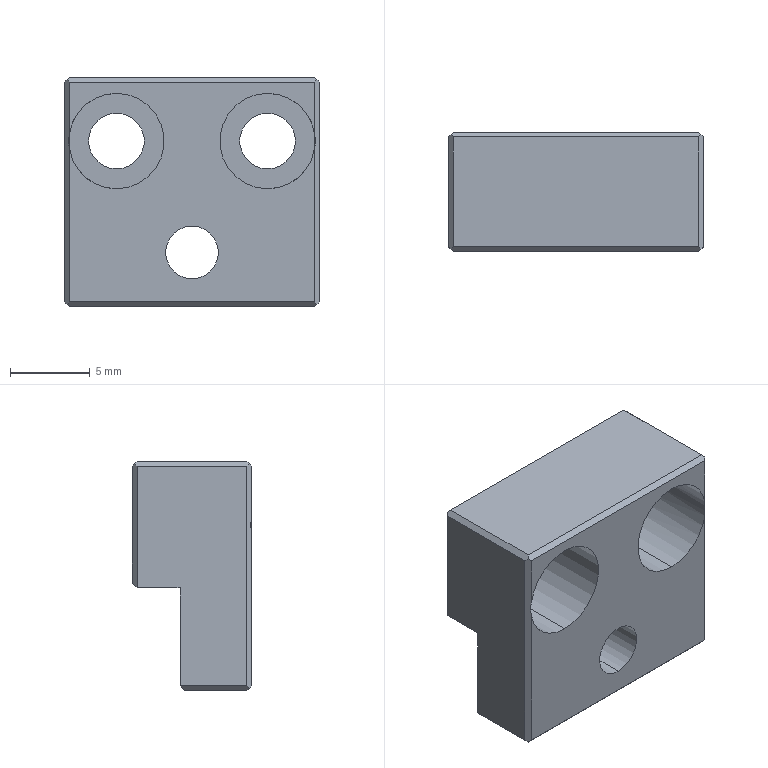Part | NX | 1 solid | 33 faces | box 16 x 7.5 x 14.4 mm | volume 1061 mm3 | plane 23 | cylinder 10 | commonest cylinder face diameters 3.5 x4 6 x4 3.3 x2
STEP:
#1=CARTESIAN_POINT('',(16.39,-63.429,11.453));
#2=VERTEX_POINT('',#1);
#3=CARTESIAN_POINT('',(0.3897,-63.429,11.453));
#4=VERTEX_POINT('',#3);
#5=CARTESIAN_POINT('',(8.39,-63.429,11.453));
#6=DIRECTION('',(-1.,0.,0.));
#7=VECTOR('',#6,1000.);
#8=LINE('',#5,#7);
#9=EDGE_CURVE('',#2,#4,#8,.T.);
#10=ORIENTED_EDGE('',*,*,#9,.F.);
#11=CARTESIAN_POINT('',(16.39,-66.129,11.453));
#12=VERTEX_POINT('',#11);
#13=CARTESIAN_POINT('',(16.39,-59.69,11.453));
#14=DIRECTION('',(0.,1.,0.));
#15=VECTOR('',#14,1000.);
#16=LINE('',#13,#15);
#17=EDGE_CURVE('',#12,#2,#16,.T.);
#18=ORIENTED_EDGE('',*,*,#17,.F.);
#19=CARTESIAN_POINT('',(0.3897,-66.129,11.453));
#20=VERTEX_POINT('',#19);
#21=CARTESIAN_POINT('',(13.89,-66.129,11.453));
#22=DIRECTION('',(-1.,0.,0.));
#23=VECTOR('',#22,1000.);
#24=LINE('',#21,#23);
#25=EDGE_CURVE('',#12,#20,#24,.T.);
#26=ORIENTED_EDGE('',*,*,#25,.T.);
#27=CARTESIAN_POINT('',(0.3897,-59.69,11.453));
#28=DIRECTION('',(0.,1.,0.));
#29=VECTOR('',#28,1000.);
#30=LINE('',#27,#29);
#31=EDGE_CURVE('',#20,#4,#30,.T.);
#32=ORIENTED_EDGE('',*,*,#31,.T.);
#33=EDGE_LOOP('',(#10,#18,#26,#32));
#34=FACE_BOUND('',#33,.T.);
#35=CARTESIAN_POINT('',(13.89,-66.629,11.453));
#36=DIRECTION('',(0.,0.,-1.));
#37=DIRECTION('',(0.,-1.,0.));
#38=AXIS2_PLACEMENT_3D('',#35,#36,#37);
#39=PLANE('',#38);
#40=ADVANCED_FACE('',(#34),#39,.T.);
#41=CARTESIAN_POINT('',(16.39,-66.129,5.303));
#42=VERTEX_POINT('',#41);
#43=CARTESIAN_POINT('',(0.3897,-66.129,5.303));
#44=VERTEX_POINT('',#43);
#45=CARTESIAN_POINT('',(8.39,-66.129,5.303));
#46=DIRECTION('',(-1.,0.,0.));
#47=VECTOR('',#46,1000.);
#48=LINE('',#45,#47);
#49=EDGE_CURVE('',#42,#44,#48,.T.);
#50=ORIENTED_EDGE('',*,*,#49,.T.);
#51=CARTESIAN_POINT('',(0.3897,-66.129,11.106));
#52=DIRECTION('',(0.,0.,-1.));
#53=VECTOR('',#52,1000.);
#54=LINE('',#51,#53);
#55=EDGE_CURVE('',#20,#44,#54,.T.);
#56=ORIENTED_EDGE('',*,*,#55,.F.);
#57=ORIENTED_EDGE('',*,*,#25,.F.);
#58=CARTESIAN_POINT('',(16.39,-66.129,11.106));
#59=DIRECTION('',(0.,0.,-1.));
#60=VECTOR('',#59,1000.);
#61=LINE('',#58,#60);
#62=EDGE_CURVE('',#12,#42,#61,.T.);
#63=ORIENTED_EDGE('',*,*,#62,.T.);
#64=EDGE_LOOP('',(#50,#56,#57,#63));
#65=FACE_BOUND('',#64,.T.);
#66=CARTESIAN_POINT('',(8.39,-66.129,6.753));
#67=VERTEX_POINT('',#66);
#68=CARTESIAN_POINT('',(8.39,-66.129,10.053));
#69=VERTEX_POINT('',#68);
#70=CARTESIAN_POINT('',(8.39,-66.129,8.403));
#71=DIRECTION('',(0.,-1.,0.));
#72=DIRECTION('',(0.,0.,1.));
#73=AXIS2_PLACEMENT_3D('',#70,#71,#72);
#74=CIRCLE('',#73,1.65);
#75=EDGE_CURVE('',#67,#69,#74,.T.);
#76=ORIENTED_EDGE('',*,*,#75,.T.);
#77=CARTESIAN_POINT('',(8.39,-66.129,8.403));
#78=DIRECTION('',(0.,-1.,0.));
#79=DIRECTION('',(0.,0.,1.));
#80=AXIS2_PLACEMENT_3D('',#77,#78,#79);
#81=CIRCLE('',#80,1.65);
#82=EDGE_CURVE('',#69,#67,#81,.T.);
#83=ORIENTED_EDGE('',*,*,#82,.T.);
#84=EDGE_LOOP('',(#76,#83));
#85=FACE_BOUND('',#84,.T.);
#86=CARTESIAN_POINT('',(13.89,-66.129,5.503));
#87=DIRECTION('',(0.,1.,0.));
#88=DIRECTION('',(1.,0.,0.));
#89=AXIS2_PLACEMENT_3D('',#86,#87,#88);
#90=PLANE('',#89);
#91=ADVANCED_FACE('',(#65,#85),#90,.T.);
#92=CARTESIAN_POINT('',(0.6897,-70.329,5.003));
#93=VERTEX_POINT('',#92);
#94=CARTESIAN_POINT('',(16.09,-70.329,5.003));
#95=VERTEX_POINT('',#94);
#96=CARTESIAN_POINT('',(8.39,-70.329,5.003));
#97=DIRECTION('',(1.,0.,0.));
#98=VECTOR('',#97,1000.);
#99=LINE('',#96,#98);
#100=EDGE_CURVE('',#93,#95,#99,.T.);
#101=ORIENTED_EDGE('',*,*,#100,.F.);
#102=CARTESIAN_POINT('',(0.6897,-66.429,5.003));
#103=VERTEX_POINT('',#102);
#104=CARTESIAN_POINT('',(0.6897,-68.379,5.003));
#105=DIRECTION('',(0.,-1.,0.));
#106=VECTOR('',#105,1000.);
#107=LINE('',#104,#106);
#108=EDGE_CURVE('',#103,#93,#107,.T.);
#109=ORIENTED_EDGE('',*,*,#108,.F.);
#110=CARTESIAN_POINT('',(16.09,-66.429,5.003));
#111=VERTEX_POINT('',#110);
#112=CARTESIAN_POINT('',(8.39,-66.429,5.003));
#113=DIRECTION('',(-1.,0.,0.));
#114=VECTOR('',#113,1000.);
#115=LINE('',#112,#114);
#116=EDGE_CURVE('',#111,#103,#115,.T.);
#117=ORIENTED_EDGE('',*,*,#116,.F.);
#118=CARTESIAN_POINT('',(16.09,-68.379,5.003));
#119=DIRECTION('',(0.,-1.,0.));
#120=VECTOR('',#119,1000.);
#121=LINE('',#118,#120);
#122=EDGE_CURVE('',#111,#95,#121,.T.);
#123=ORIENTED_EDGE('',*,*,#122,.T.);
#124=EDGE_LOOP('',(#101,#109,#117,#123));
#125=FACE_BOUND('',#124,.T.);
#126=CARTESIAN_POINT('',(13.89,-70.329,5.003));
#127=DIRECTION('',(0.,0.,-1.));
#128=DIRECTION('',(0.,-1.,0.));
#129=AXIS2_PLACEMENT_3D('',#126,#127,#128);
#130=PLANE('',#129);
#131=ADVANCED_FACE('',(#125),#130,.T.);
#132=CARTESIAN_POINT('',(16.09,-70.629,19.103));
#133=VERTEX_POINT('',#132);
#134=CARTESIAN_POINT('',(0.6897,-70.629,19.103));
#135=VERTEX_POINT('',#134);
#136=CARTESIAN_POINT('',(8.39,-70.629,19.103));
#137=DIRECTION('',(-1.,0.,0.));
#138=VECTOR('',#137,1000.);
#139=LINE('',#136,#138);
#140=EDGE_CURVE('',#133,#135,#139,.T.);
#141=ORIENTED_EDGE('',*,*,#140,.T.);
#142=CARTESIAN_POINT('',(0.6897,-70.629,15.949));
#143=VERTEX_POINT('',#142);
#144=CARTESIAN_POINT('',(0.6897,-70.629,11.106));
#145=DIRECTION('',(0.,0.,-1.));
#146=VECTOR('',#145,1000.);
#147=LINE('',#144,#146);
#148=EDGE_CURVE('',#135,#143,#147,.T.);
#149=ORIENTED_EDGE('',*,*,#148,.T.);
#150=CARTESIAN_POINT('',(3.64,-70.629,18.403));
#151=VERTEX_POINT('',#150);
#152=CARTESIAN_POINT('',(3.64,-70.629,15.403));
#153=DIRECTION('',(0.,-1.,0.));
#154=DIRECTION('',(0.,0.,1.));
#155=AXIS2_PLACEMENT_3D('',#152,#153,#154);
#156=CIRCLE('',#155,3.);
#157=EDGE_CURVE('',#151,#143,#156,.T.);
#158=ORIENTED_EDGE('',*,*,#157,.F.);
#159=CARTESIAN_POINT('',(3.64,-70.629,12.403));
#160=VERTEX_POINT('',#159);
#161=CARTESIAN_POINT('',(3.64,-70.629,15.403));
#162=DIRECTION('',(0.,-1.,0.));
#163=DIRECTION('',(0.,0.,1.));
#164=AXIS2_PLACEMENT_3D('',#161,#162,#163);
#165=CIRCLE('',#164,3.);
#166=EDGE_CURVE('',#160,#151,#165,.T.);
#167=ORIENTED_EDGE('',*,*,#166,.F.);
#168=CARTESIAN_POINT('',(0.6897,-70.629,14.858));
#169=VERTEX_POINT('',#168);
#170=CARTESIAN_POINT('',(3.64,-70.629,15.403));
#171=DIRECTION('',(0.,-1.,0.));
#172=DIRECTION('',(0.,0.,1.));
#173=AXIS2_PLACEMENT_3D('',#170,#171,#172);
#174=CIRCLE('',#173,3.);
#175=EDGE_CURVE('',#169,#160,#174,.T.);
#176=ORIENTED_EDGE('',*,*,#175,.F.);
#177=CARTESIAN_POINT('',(0.6897,-70.629,5.303));
#178=VERTEX_POINT('',#177);
#179=CARTESIAN_POINT('',(0.6897,-70.629,11.106));
#180=DIRECTION('',(0.,0.,-1.));
#181=VECTOR('',#180,1000.);
#182=LINE('',#179,#181);
#183=EDGE_CURVE('',#169,#178,#182,.T.);
#184=ORIENTED_EDGE('',*,*,#183,.T.);
#185=CARTESIAN_POINT('',(16.09,-70.629,5.303));
#186=VERTEX_POINT('',#185);
#187=CARTESIAN_POINT('',(8.39,-70.629,5.303));
#188=DIRECTION('',(1.,0.,0.));
#189=VECTOR('',#188,1000.);
#190=LINE('',#187,#189);
#191=EDGE_CURVE('',#178,#186,#190,.T.);
#192=ORIENTED_EDGE('',*,*,#191,.T.);
#193=CARTESIAN_POINT('',(16.09,-70.629,14.858));
#194=VERTEX_POINT('',#193);
#195=CARTESIAN_POINT('',(16.09,-70.629,11.106));
#196=DIRECTION('',(0.,0.,-1.));
#197=VECTOR('',#196,1000.);
#198=LINE('',#195,#197);
#199=EDGE_CURVE('',#194,#186,#198,.T.);
#200=ORIENTED_EDGE('',*,*,#199,.F.);
#201=CARTESIAN_POINT('',(13.14,-70.629,12.403));
#202=VERTEX_POINT('',#201);
#203=CARTESIAN_POINT('',(13.14,-70.629,15.403));
#204=DIRECTION('',(0.,-1.,0.));
#205=DIRECTION('',(0.,0.,1.));
#206=AXIS2_PLACEMENT_3D('',#203,#204,#205);
#207=CIRCLE('',#206,3.);
#208=EDGE_CURVE('',#202,#194,#207,.T.);
#209=ORIENTED_EDGE('',*,*,#208,.F.);
#210=CARTESIAN_POINT('',(13.14,-70.629,18.403));
#211=VERTEX_POINT('',#210);
#212=CARTESIAN_POINT('',(13.14,-70.629,15.403));
#213=DIRECTION('',(0.,-1.,0.));
#214=DIRECTION('',(0.,0.,1.));
#215=AXIS2_PLACEMENT_3D('',#212,#213,#214);
#216=CIRCLE('',#215,3.);
#217=EDGE_CURVE('',#211,#202,#216,.T.);
#218=ORIENTED_EDGE('',*,*,#217,.F.);
#219=CARTESIAN_POINT('',(16.09,-70.629,15.949));
#220=VERTEX_POINT('',#219);
#221=CARTESIAN_POINT('',(13.14,-70.629,15.403));
#222=DIRECTION('',(0.,-1.,0.));
#223=DIRECTION('',(0.,0.,1.));
#224=AXIS2_PLACEMENT_3D('',#221,#222,#223);
#225=CIRCLE('',#224,3.);
#226=EDGE_CURVE('',#220,#211,#225,.T.);
#227=ORIENTED_EDGE('',*,*,#226,.F.);
#228=CARTESIAN_POINT('',(16.09,-70.629,11.106));
#229=DIRECTION('',(0.,0.,-1.));
#230=VECTOR('',#229,1000.);
#231=LINE('',#228,#230);
#232=EDGE_CURVE('',#133,#220,#231,.T.);
#233=ORIENTED_EDGE('',*,*,#232,.F.);
#234=EDGE_LOOP('',(#141,#149,#158,#167,#176,#184,#192,#200,#209,#218,#227,#233));
#235=FACE_BOUND('',#234,.T.);
#236=CARTESIAN_POINT('',(8.39,-70.629,6.753));
#237=VERTEX_POINT('',#236);
#238=CARTESIAN_POINT('',(8.39,-70.629,10.053));
#239=VERTEX_POINT('',#238);
#240=CARTESIAN_POINT('',(8.39,-70.629,8.403));
#241=DIRECTION('',(0.,-1.,0.));
#242=DIRECTION('',(0.,0.,1.));
#243=AXIS2_PLACEMENT_3D('',#240,#241,#242);
#244=CIRCLE('',#243,1.65);
#245=EDGE_CURVE('',#237,#239,#244,.T.);
#246=ORIENTED_EDGE('',*,*,#245,.F.);
#247=CARTESIAN_POINT('',(8.39,-70.629,8.403));
#248=DIRECTION('',(0.,-1.,0.));
#249=DIRECTION('',(0.,0.,1.));
#250=AXIS2_PLACEMENT_3D('',#247,#248,#249);
#251=CIRCLE('',#250,1.65);
#252=EDGE_CURVE('',#239,#237,#251,.T.);
#253=ORIENTED_EDGE('',*,*,#252,.F.);
#254=EDGE_LOOP('',(#246,#253));
#255=FACE_BOUND('',#254,.T.);
#256=CARTESIAN_POINT('',(13.89,-70.629,20.403));
#257=DIRECTION('',(0.,-1.,0.));
#258=DIRECTION('',(-1.,0.,0.));
#259=AXIS2_PLACEMENT_3D('',#256,#257,#258);
#260=PLANE('',#259);
#261=ADVANCED_FACE('',(#235,#255),#260,.T.);
#262=CARTESIAN_POINT('',(0.6897,-63.429,19.403));
#263=VERTEX_POINT('',#262);
#264=CARTESIAN_POINT('',(16.09,-63.429,19.403));
#265=VERTEX_POINT('',#264);
#266=CARTESIAN_POINT('',(8.39,-63.429,19.403));
#267=DIRECTION('',(1.,0.,0.));
#268=VECTOR('',#267,1000.);
#269=LINE('',#266,#268);
#270=EDGE_CURVE('',#263,#265,#269,.T.);
#271=ORIENTED_EDGE('',*,*,#270,.F.);
#272=CARTESIAN_POINT('',(0.6897,-70.329,19.403));
#273=VERTEX_POINT('',#272);
#274=CARTESIAN_POINT('',(0.6897,-66.879,19.403));
#275=DIRECTION('',(0.,1.,0.));
#276=VECTOR('',#275,1000.);
#277=LINE('',#274,#276);
#278=EDGE_CURVE('',#273,#263,#277,.T.);
#279=ORIENTED_EDGE('',*,*,#278,.F.);
#280=CARTESIAN_POINT('',(16.09,-70.329,19.403));
#281=VERTEX_POINT('',#280);
#282=CARTESIAN_POINT('',(8.39,-70.329,19.403));
#283=DIRECTION('',(-1.,0.,0.));
#284=VECTOR('',#283,1000.);
#285=LINE('',#282,#284);
#286=EDGE_CURVE('',#281,#273,#285,.T.);
#287=ORIENTED_EDGE('',*,*,#286,.F.);
#288=CARTESIAN_POINT('',(16.09,-66.879,19.403));
#289=DIRECTION('',(0.,1.,0.));
#290=VECTOR('',#289,1000.);
#291=LINE('',#288,#290);
#292=EDGE_CURVE('',#281,#265,#291,.T.);
#293=ORIENTED_EDGE('',*,*,#292,.T.);
#294=EDGE_LOOP('',(#271,#279,#287,#293));
#295=FACE_BOUND('',#294,.T.);
#296=CARTESIAN_POINT('',(13.89,-63.129,19.403));
#297=DIRECTION('',(0.,0.,1.));
#298=DIRECTION('',(1.,0.,0.));
#299=AXIS2_PLACEMENT_3D('',#296,#297,#298);
#300=PLANE('',#299);
#301=ADVANCED_FACE('',(#295),#300,.T.);
#302=CARTESIAN_POINT('',(16.09,-63.129,19.103));
#303=VERTEX_POINT('',#302);
#304=CARTESIAN_POINT('',(16.09,-63.129,11.753));
#305=VERTEX_POINT('',#304);
#306=CARTESIAN_POINT('',(16.09,-63.129,15.428));
#307=DIRECTION('',(0.,0.,-1.));
#308=VECTOR('',#307,1000.);
#309=LINE('',#306,#308);
#310=EDGE_CURVE('',#303,#305,#309,.T.);
#311=ORIENTED_EDGE('',*,*,#310,.T.);
#312=CARTESIAN_POINT('',(0.6897,-63.129,11.753));
#313=VERTEX_POINT('',#312);
#314=CARTESIAN_POINT('',(8.39,-63.129,11.753));
#315=DIRECTION('',(-1.,0.,0.));
#316=VECTOR('',#315,1000.);
#317=LINE('',#314,#316);
#318=EDGE_CURVE('',#305,#313,#317,.T.);
#319=ORIENTED_EDGE('',*,*,#318,.T.);
#320=CARTESIAN_POINT('',(0.6897,-63.129,19.103));
#321=VERTEX_POINT('',#320);
#322=CARTESIAN_POINT('',(0.6897,-63.129,15.428));
#323=DIRECTION('',(0.,0.,-1.));
#324=VECTOR('',#323,1000.);
#325=LINE('',#322,#324);
#326=EDGE_CURVE('',#321,#313,#325,.T.);
#327=ORIENTED_EDGE('',*,*,#326,.F.);
#328=CARTESIAN_POINT('',(8.39,-63.129,19.103));
#329=DIRECTION('',(1.,0.,0.));
#330=VECTOR('',#329,1000.);
#331=LINE('',#328,#330);
#332=EDGE_CURVE('',#321,#303,#331,.T.);
#333=ORIENTED_EDGE('',*,*,#332,.T.);
#334=EDGE_LOOP('',(#311,#319,#327,#333));
#335=FACE_BOUND('',#334,.T.);
#336=CARTESIAN_POINT('',(3.64,-63.129,13.653));
#337=VERTEX_POINT('',#336);
#338=CARTESIAN_POINT('',(3.64,-63.129,17.153));
#339=VERTEX_POINT('',#338);
#340=CARTESIAN_POINT('',(3.64,-63.129,15.403));
#341=DIRECTION('',(0.,-1.,0.));
#342=DIRECTION('',(0.,0.,1.));
#343=AXIS2_PLACEMENT_3D('',#340,#341,#342);
#344=CIRCLE('',#343,1.75);
#345=EDGE_CURVE('',#337,#339,#344,.T.);
#346=ORIENTED_EDGE('',*,*,#345,.T.);
#347=CARTESIAN_POINT('',(3.64,-63.129,15.403));
#348=DIRECTION('',(0.,-1.,0.));
#349=DIRECTION('',(0.,0.,1.));
#350=AXIS2_PLACEMENT_3D('',#347,#348,#349);
#351=CIRCLE('',#350,1.75);
#352=EDGE_CURVE('',#339,#337,#351,.T.);
#353=ORIENTED_EDGE('',*,*,#352,.T.);
#354=EDGE_LOOP('',(#346,#353));
#355=FACE_BOUND('',#354,.T.);
#356=CARTESIAN_POINT('',(13.14,-63.129,13.653));
#357=VERTEX_POINT('',#356);
#358=CARTESIAN_POINT('',(13.14,-63.129,17.153));
#359=VERTEX_POINT('',#358);
#360=CARTESIAN_POINT('',(13.14,-63.129,15.403));
#361=DIRECTION('',(0.,-1.,0.));
#362=DIRECTION('',(0.,0.,1.));
#363=AXIS2_PLACEMENT_3D('',#360,#361,#362);
#364=CIRCLE('',#363,1.75);
#365=EDGE_CURVE('',#357,#359,#364,.T.);
#366=ORIENTED_EDGE('',*,*,#365,.T.);
#367=CARTESIAN_POINT('',(13.14,-63.129,15.403));
#368=DIRECTION('',(0.,-1.,0.));
#369=DIRECTION('',(0.,0.,1.));
#370=AXIS2_PLACEMENT_3D('',#367,#368,#369);
#371=CIRCLE('',#370,1.75);
#372=EDGE_CURVE('',#359,#357,#371,.T.);
#373=ORIENTED_EDGE('',*,*,#372,.T.);
#374=EDGE_LOOP('',(#366,#373));
#375=FACE_BOUND('',#374,.T.);
#376=CARTESIAN_POINT('',(13.89,-63.129,11.253));
#377=DIRECTION('',(0.,1.,0.));
#378=DIRECTION('',(1.,0.,0.));
#379=AXIS2_PLACEMENT_3D('',#376,#377,#378);
#380=PLANE('',#379);
#381=ADVANCED_FACE('',(#335,#355,#375),#380,.T.);
#382=ORIENTED_EDGE('',*,*,#157,.T.);
#383=CARTESIAN_POINT('',(0.6897,-70.629,15.949));
#384=CARTESIAN_POINT('',(0.6229,-70.562,15.587));
#385=CARTESIAN_POINT('',(0.6229,-70.562,15.219));
#386=CARTESIAN_POINT('',(0.6897,-70.629,14.858));
#387=(BOUNDED_CURVE()B_SPLINE_CURVE(3,(#383,#384,#385,#386),.UNSPECIFIED.,.F.,.F.)B_SPLINE_CURVE_WITH_KNOTS((4,4),(2.959,3.324),.UNSPECIFIED.)CURVE()GEOMETRIC_REPRESENTATION_ITEM()RATIONAL_B_SPLINE_CURVE((1.,0.9889,0.9889,1.))REPRESENTATION_ITEM(''));
#388=EDGE_CURVE('',#143,#169,#387,.T.);
#389=ORIENTED_EDGE('',*,*,#388,.T.);
#390=ORIENTED_EDGE('',*,*,#175,.T.);
#391=CARTESIAN_POINT('',(3.64,-66.129,12.403));
#392=VERTEX_POINT('',#391);
#393=CARTESIAN_POINT('',(3.64,-69.629,12.403));
#394=DIRECTION('',(0.,-1.,0.));
#395=VECTOR('',#394,1000.);
#396=LINE('',#393,#395);
#397=EDGE_CURVE('',#160,#392,#396,.F.);
#398=ORIENTED_EDGE('',*,*,#397,.T.);
#399=CARTESIAN_POINT('',(3.64,-66.129,18.403));
#400=VERTEX_POINT('',#399);
#401=CARTESIAN_POINT('',(3.64,-66.129,15.403));
#402=DIRECTION('',(0.,-1.,0.));
#403=DIRECTION('',(0.,0.,1.));
#404=AXIS2_PLACEMENT_3D('',#401,#402,#403);
#405=CIRCLE('',#404,3.);
#406=EDGE_CURVE('',#400,#392,#405,.T.);
#407=ORIENTED_EDGE('',*,*,#406,.F.);
#408=CARTESIAN_POINT('',(3.64,-69.629,18.403));
#409=DIRECTION('',(0.,-1.,0.));
#410=VECTOR('',#409,1000.);
#411=LINE('',#408,#410);
#412=EDGE_CURVE('',#151,#400,#411,.F.);
#413=ORIENTED_EDGE('',*,*,#412,.F.);
#414=EDGE_LOOP('',(#382,#389,#390,#398,#407,#413));
#415=FACE_BOUND('',#414,.T.);
#416=CARTESIAN_POINT('',(3.64,-69.629,15.403));
#417=DIRECTION('',(0.,-1.,0.));
#418=DIRECTION('',(0.,0.,1.));
#419=AXIS2_PLACEMENT_3D('',#416,#417,#418);
#420=CYLINDRICAL_SURFACE('',#419,3.);
#421=ADVANCED_FACE('',(#415),#420,.F.);
#422=CARTESIAN_POINT('',(3.64,-66.129,15.403));
#423=DIRECTION('',(0.,-1.,0.));
#424=DIRECTION('',(0.,0.,1.));
#425=AXIS2_PLACEMENT_3D('',#422,#423,#424);
#426=CIRCLE('',#425,3.);
#427=EDGE_CURVE('',#392,#400,#426,.T.);
#428=ORIENTED_EDGE('',*,*,#427,.T.);
#429=ORIENTED_EDGE('',*,*,#406,.T.);
#430=EDGE_LOOP('',(#428,#429));
#431=FACE_BOUND('',#430,.T.);
#432=CARTESIAN_POINT('',(3.64,-66.129,13.653));
#433=VERTEX_POINT('',#432);
#434=CARTESIAN_POINT('',(3.64,-66.129,17.153));
#435=VERTEX_POINT('',#434);
#436=CARTESIAN_POINT('',(3.64,-66.129,15.403));
#437=DIRECTION('',(0.,-1.,0.));
#438=DIRECTION('',(0.,0.,1.));
#439=AXIS2_PLACEMENT_3D('',#436,#437,#438);
#440=CIRCLE('',#439,1.75);
#441=EDGE_CURVE('',#433,#435,#440,.T.);
#442=ORIENTED_EDGE('',*,*,#441,.F.);
#443=CARTESIAN_POINT('',(3.64,-66.129,15.403));
#444=DIRECTION('',(0.,-1.,0.));
#445=DIRECTION('',(0.,0.,1.));
#446=AXIS2_PLACEMENT_3D('',#443,#444,#445);
#447=CIRCLE('',#446,1.75);
#448=EDGE_CURVE('',#435,#433,#447,.T.);
#449=ORIENTED_EDGE('',*,*,#448,.F.);
#450=EDGE_LOOP('',(#442,#449));
#451=FACE_BOUND('',#450,.T.);
#452=CARTESIAN_POINT('',(3.64,-66.129,15.403));
#453=DIRECTION('',(0.,-1.,0.));
#454=DIRECTION('',(-1.,0.,0.));
#455=AXIS2_PLACEMENT_3D('',#452,#453,#454);
#456=PLANE('',#455);
#457=ADVANCED_FACE('',(#431,#451),#456,.T.);
#458=ORIENTED_EDGE('',*,*,#441,.T.);
#459=CARTESIAN_POINT('',(3.64,-69.629,17.153));
#460=DIRECTION('',(0.,-1.,0.));
#461=VECTOR('',#460,1000.);
#462=LINE('',#459,#461);
#463=EDGE_CURVE('',#339,#435,#462,.T.);
#464=ORIENTED_EDGE('',*,*,#463,.F.);
#465=ORIENTED_EDGE('',*,*,#345,.F.);
#466=CARTESIAN_POINT('',(3.64,-69.629,13.653));
#467=DIRECTION('',(0.,-1.,0.));
#468=VECTOR('',#467,1000.);
#469=LINE('',#466,#468);
#470=EDGE_CURVE('',#337,#433,#469,.T.);
#471=ORIENTED_EDGE('',*,*,#470,.T.);
#472=EDGE_LOOP('',(#458,#464,#465,#471));
#473=FACE_BOUND('',#472,.T.);
#474=CARTESIAN_POINT('',(3.64,-69.629,15.403));
#475=DIRECTION('',(0.,-1.,0.));
#476=DIRECTION('',(0.,0.,1.));
#477=AXIS2_PLACEMENT_3D('',#474,#475,#476);
#478=CYLINDRICAL_SURFACE('',#477,1.75);
#479=ADVANCED_FACE('',(#473),#478,.F.);
#480=CARTESIAN_POINT('',(13.14,-66.129,13.653));
#481=VERTEX_POINT('',#480);
#482=CARTESIAN_POINT('',(13.14,-66.129,17.153));
#483=VERTEX_POINT('',#482);
#484=CARTESIAN_POINT('',(13.14,-66.129,15.403));
#485=DIRECTION('',(0.,-1.,0.));
#486=DIRECTION('',(0.,0.,1.));
#487=AXIS2_PLACEMENT_3D('',#484,#485,#486);
#488=CIRCLE('',#487,1.75);
#489=EDGE_CURVE('',#481,#483,#488,.T.);
#490=ORIENTED_EDGE('',*,*,#489,.T.);
#491=CARTESIAN_POINT('',(13.14,-69.629,17.153));
#492=DIRECTION('',(0.,-1.,0.));
#493=VECTOR('',#492,1000.);
#494=LINE('',#491,#493);
#495=EDGE_CURVE('',#483,#359,#494,.F.);
#496=ORIENTED_EDGE('',*,*,#495,.T.);
#497=ORIENTED_EDGE('',*,*,#365,.F.);
#498=CARTESIAN_POINT('',(13.14,-69.629,13.653));
#499=DIRECTION('',(0.,-1.,0.));
#500=VECTOR('',#499,1000.);
#501=LINE('',#498,#500);
#502=EDGE_CURVE('',#481,#357,#501,.F.);
#503=ORIENTED_EDGE('',*,*,#502,.F.);
#504=EDGE_LOOP('',(#490,#496,#497,#503));
#505=FACE_BOUND('',#504,.T.);
#506=CARTESIAN_POINT('',(13.14,-69.629,15.403));
#507=DIRECTION('',(0.,-1.,0.));
#508=DIRECTION('',(0.,0.,1.));
#509=AXIS2_PLACEMENT_3D('',#506,#507,#508);
#510=CYLINDRICAL_SURFACE('',#509,1.75);
#511=ADVANCED_FACE('',(#505),#510,.F.);
#512=CARTESIAN_POINT('',(13.14,-66.129,12.403));
#513=VERTEX_POINT('',#512);
#514=CARTESIAN_POINT('',(13.14,-66.129,18.403));
#515=VERTEX_POINT('',#514);
#516=CARTESIAN_POINT('',(13.14,-66.129,15.403));
#517=DIRECTION('',(0.,-1.,0.));
#518=DIRECTION('',(0.,0.,1.));
#519=AXIS2_PLACEMENT_3D('',#516,#517,#518);
#520=CIRCLE('',#519,3.);
#521=EDGE_CURVE('',#513,#515,#520,.T.);
#522=ORIENTED_EDGE('',*,*,#521,.T.);
#523=CARTESIAN_POINT('',(13.14,-66.129,15.403));
#524=DIRECTION('',(0.,-1.,0.));
#525=DIRECTION('',(0.,0.,1.));
#526=AXIS2_PLACEMENT_3D('',#523,#524,#525);
#527=CIRCLE('',#526,3.);
#528=EDGE_CURVE('',#515,#513,#527,.T.);
#529=ORIENTED_EDGE('',*,*,#528,.T.);
#530=EDGE_LOOP('',(#522,#529));
#531=FACE_BOUND('',#530,.T.);
#532=ORIENTED_EDGE('',*,*,#489,.F.);
#533=CARTESIAN_POINT('',(13.14,-66.129,15.403));
#534=DIRECTION('',(0.,-1.,0.));
#535=DIRECTION('',(0.,0.,1.));
#536=AXIS2_PLACEMENT_3D('',#533,#534,#535);
#537=CIRCLE('',#536,1.75);
#538=EDGE_CURVE('',#483,#481,#537,.T.);
#539=ORIENTED_EDGE('',*,*,#538,.F.);
#540=EDGE_LOOP('',(#532,#539));
#541=FACE_BOUND('',#540,.T.);
#542=CARTESIAN_POINT('',(13.14,-66.129,15.403));
#543=DIRECTION('',(0.,-1.,0.));
#544=DIRECTION('',(-1.,0.,0.));
#545=AXIS2_PLACEMENT_3D('',#542,#543,#544);
#546=PLANE('',#545);
#547=ADVANCED_FACE('',(#531,#541),#546,.T.);
#548=ORIENTED_EDGE('',*,*,#208,.T.);
#549=CARTESIAN_POINT('',(16.09,-70.629,15.949));
#550=CARTESIAN_POINT('',(16.157,-70.562,15.587));
#551=CARTESIAN_POINT('',(16.157,-70.562,15.219));
#552=CARTESIAN_POINT('',(16.09,-70.629,14.858));
#553=(BOUNDED_CURVE()B_SPLINE_CURVE(3,(#549,#550,#551,#552),.UNSPECIFIED.,.F.,.F.)B_SPLINE_CURVE_WITH_KNOTS((4,4),(2.959,3.324),.UNSPECIFIED.)CURVE()GEOMETRIC_REPRESENTATION_ITEM()RATIONAL_B_SPLINE_CURVE((1.,0.9889,0.9889,1.))REPRESENTATION_ITEM(''));
#554=EDGE_CURVE('',#220,#194,#553,.T.);
#555=ORIENTED_EDGE('',*,*,#554,.F.);
#556=ORIENTED_EDGE('',*,*,#226,.T.);
#557=CARTESIAN_POINT('',(13.14,-69.629,18.403));
#558=DIRECTION('',(0.,-1.,0.));
#559=VECTOR('',#558,1000.);
#560=LINE('',#557,#559);
#561=EDGE_CURVE('',#515,#211,#560,.T.);
#562=ORIENTED_EDGE('',*,*,#561,.F.);
#563=ORIENTED_EDGE('',*,*,#521,.F.);
#564=CARTESIAN_POINT('',(13.14,-69.629,12.403));
#565=DIRECTION('',(0.,-1.,0.));
#566=VECTOR('',#565,1000.);
#567=LINE('',#564,#566);
#568=EDGE_CURVE('',#513,#202,#567,.T.);
#569=ORIENTED_EDGE('',*,*,#568,.T.);
#570=EDGE_LOOP('',(#548,#555,#556,#562,#563,#569));
#571=FACE_BOUND('',#570,.T.);
#572=CARTESIAN_POINT('',(13.14,-69.629,15.403));
#573=DIRECTION('',(0.,-1.,0.));
#574=DIRECTION('',(0.,0.,1.));
#575=AXIS2_PLACEMENT_3D('',#572,#573,#574);
#576=CYLINDRICAL_SURFACE('',#575,3.);
#577=ADVANCED_FACE('',(#571),#576,.F.);
#578=ORIENTED_EDGE('',*,*,#245,.T.);
#579=CARTESIAN_POINT('',(8.39,-69.629,10.053));
#580=DIRECTION('',(0.,-1.,0.));
#581=VECTOR('',#580,1000.);
#582=LINE('',#579,#581);
#583=EDGE_CURVE('',#69,#239,#582,.T.);
#584=ORIENTED_EDGE('',*,*,#583,.F.);
#585=ORIENTED_EDGE('',*,*,#75,.F.);
#586=CARTESIAN_POINT('',(8.39,-69.629,6.753));
#587=DIRECTION('',(0.,-1.,0.));
#588=VECTOR('',#587,1000.);
#589=LINE('',#586,#588);
#590=EDGE_CURVE('',#67,#237,#589,.T.);
#591=ORIENTED_EDGE('',*,*,#590,.T.);
#592=EDGE_LOOP('',(#578,#584,#585,#591));
#593=FACE_BOUND('',#592,.T.);
#594=CARTESIAN_POINT('',(8.39,-69.629,8.403));
#595=DIRECTION('',(0.,-1.,0.));
#596=DIRECTION('',(0.,0.,1.));
#597=AXIS2_PLACEMENT_3D('',#594,#595,#596);
#598=CYLINDRICAL_SURFACE('',#597,1.65);
#599=ADVANCED_FACE('',(#593),#598,.F.);
#600=ORIENTED_EDGE('',*,*,#140,.F.);
#601=CARTESIAN_POINT('',(16.24,-70.479,19.253));
#602=VERTEX_POINT('',#601);
#603=CARTESIAN_POINT('',(27.028,-59.69,30.042));
#604=DIRECTION('',(0.5774,0.5774,0.5774));
#605=VECTOR('',#604,1000.);
#606=LINE('',#603,#605);
#607=EDGE_CURVE('',#133,#602,#606,.T.);
#608=ORIENTED_EDGE('',*,*,#607,.T.);
#609=CARTESIAN_POINT('',(5.451,-59.69,30.042));
#610=DIRECTION('',(-0.5774,0.5774,0.5774));
#611=VECTOR('',#610,1000.);
#612=LINE('',#609,#611);
#613=EDGE_CURVE('',#602,#281,#612,.T.);
#614=ORIENTED_EDGE('',*,*,#613,.T.);
#615=ORIENTED_EDGE('',*,*,#286,.T.);
#616=CARTESIAN_POINT('',(0.5397,-70.479,19.253));
#617=VERTEX_POINT('',#616);
#618=CARTESIAN_POINT('',(13.89,-57.129,32.603));
#619=DIRECTION('',(-0.5774,-0.5774,-0.5774));
#620=VECTOR('',#619,1000.);
#621=LINE('',#618,#620);
#622=EDGE_CURVE('',#273,#617,#621,.T.);
#623=ORIENTED_EDGE('',*,*,#622,.T.);
#624=CARTESIAN_POINT('',(13.89,-83.829,5.903));
#625=DIRECTION('',(0.5774,-0.5774,-0.5774));
#626=VECTOR('',#625,1000.);
#627=LINE('',#624,#626);
#628=EDGE_CURVE('',#617,#135,#627,.T.);
#629=ORIENTED_EDGE('',*,*,#628,.T.);
#630=EDGE_LOOP('',(#600,#608,#614,#615,#623,#629));
#631=FACE_BOUND('',#630,.T.);
#632=CARTESIAN_POINT('',(8.39,-70.479,19.253));
#633=DIRECTION('',(0.,-0.7071,0.7071));
#634=DIRECTION('',(-1.,0.,0.));
#635=AXIS2_PLACEMENT_3D('',#632,#633,#634);
#636=PLANE('',#635);
#637=ADVANCED_FACE('',(#631),#636,.T.);
#638=ORIENTED_EDGE('',*,*,#270,.T.);
#639=CARTESIAN_POINT('',(16.24,-63.279,19.253));
#640=VERTEX_POINT('',#639);
#641=CARTESIAN_POINT('',(13.89,-65.629,21.603));
#642=DIRECTION('',(-0.5774,-0.5774,0.5774));
#643=VECTOR('',#642,1000.);
#644=LINE('',#641,#643);
#645=EDGE_CURVE('',#640,#265,#644,.T.);
#646=ORIENTED_EDGE('',*,*,#645,.F.);
#647=CARTESIAN_POINT('',(13.89,-60.929,16.903));
#648=DIRECTION('',(-0.5774,0.5774,-0.5774));
#649=VECTOR('',#648,1000.);
#650=LINE('',#647,#649);
#651=EDGE_CURVE('',#640,#303,#650,.T.);
#652=ORIENTED_EDGE('',*,*,#651,.T.);
#653=ORIENTED_EDGE('',*,*,#332,.F.);
#654=CARTESIAN_POINT('',(0.5397,-63.279,19.253));
#655=VERTEX_POINT('',#654);
#656=CARTESIAN_POINT('',(13.89,-49.929,5.903));
#657=DIRECTION('',(0.5774,0.5774,-0.5774));
#658=VECTOR('',#657,1000.);
#659=LINE('',#656,#658);
#660=EDGE_CURVE('',#655,#321,#659,.T.);
#661=ORIENTED_EDGE('',*,*,#660,.F.);
#662=CARTESIAN_POINT('',(13.89,-76.629,32.603));
#663=DIRECTION('',(0.5774,-0.5774,0.5774));
#664=VECTOR('',#663,1000.);
#665=LINE('',#662,#664);
#666=EDGE_CURVE('',#655,#263,#665,.T.);
#667=ORIENTED_EDGE('',*,*,#666,.T.);
#668=EDGE_LOOP('',(#638,#646,#652,#653,#661,#667));
#669=FACE_BOUND('',#668,.T.);
#670=CARTESIAN_POINT('',(8.39,-63.279,19.253));
#671=DIRECTION('',(0.,-0.7071,-0.7071));
#672=DIRECTION('',(0.,-0.7071,0.7071));
#673=AXIS2_PLACEMENT_3D('',#670,#671,#672);
#674=PLANE('',#673);
#675=ADVANCED_FACE('',(#669),#674,.F.);
#676=ORIENTED_EDGE('',*,*,#100,.T.);
#677=CARTESIAN_POINT('',(16.24,-70.479,5.153));
#678=VERTEX_POINT('',#677);
#679=CARTESIAN_POINT('',(5.451,-59.69,-5.635));
#680=DIRECTION('',(-0.5774,0.5774,-0.5774));
#681=VECTOR('',#680,1000.);
#682=LINE('',#679,#681);
#683=EDGE_CURVE('',#678,#95,#682,.T.);
#684=ORIENTED_EDGE('',*,*,#683,.F.);
#685=CARTESIAN_POINT('',(27.028,-59.69,-5.635));
#686=DIRECTION('',(0.5774,0.5774,-0.5774));
#687=VECTOR('',#686,1000.);
#688=LINE('',#685,#687);
#689=EDGE_CURVE('',#186,#678,#688,.T.);
#690=ORIENTED_EDGE('',*,*,#689,.F.);
#691=ORIENTED_EDGE('',*,*,#191,.F.);
#692=CARTESIAN_POINT('',(0.5397,-70.479,5.153));
#693=VERTEX_POINT('',#692);
#694=CARTESIAN_POINT('',(13.89,-83.829,18.503));
#695=DIRECTION('',(-0.5774,0.5774,-0.5774));
#696=VECTOR('',#695,1000.);
#697=LINE('',#694,#696);
#698=EDGE_CURVE('',#178,#693,#697,.T.);
#699=ORIENTED_EDGE('',*,*,#698,.T.);
#700=CARTESIAN_POINT('',(11.328,-59.69,-5.635));
#701=DIRECTION('',(-0.5774,-0.5774,0.5774));
#702=VECTOR('',#701,1000.);
#703=LINE('',#700,#702);
#704=EDGE_CURVE('',#93,#693,#703,.T.);
#705=ORIENTED_EDGE('',*,*,#704,.F.);
#706=EDGE_LOOP('',(#676,#684,#690,#691,#699,#705));
#707=FACE_BOUND('',#706,.T.);
#708=CARTESIAN_POINT('',(8.39,-70.479,5.153));
#709=DIRECTION('',(0.,0.7071,0.7071));
#710=DIRECTION('',(1.,0.,0.));
#711=AXIS2_PLACEMENT_3D('',#708,#709,#710);
#712=PLANE('',#711);
#713=ADVANCED_FACE('',(#707),#712,.F.);
#714=ORIENTED_EDGE('',*,*,#49,.F.);
#715=CARTESIAN_POINT('',(13.89,-68.629,2.803));
#716=DIRECTION('',(-0.5774,-0.5774,-0.5774));
#717=VECTOR('',#716,1000.);
#718=LINE('',#715,#717);
#719=EDGE_CURVE('',#42,#111,#718,.T.);
#720=ORIENTED_EDGE('',*,*,#719,.T.);
#721=ORIENTED_EDGE('',*,*,#116,.T.);
#722=CARTESIAN_POINT('',(13.89,-79.629,-8.197));
#723=DIRECTION('',(-0.5774,0.5774,0.5774));
#724=VECTOR('',#723,1000.);
#725=LINE('',#722,#724);
#726=EDGE_CURVE('',#103,#44,#725,.T.);
#727=ORIENTED_EDGE('',*,*,#726,.T.);
#728=EDGE_LOOP('',(#714,#720,#721,#727));
#729=FACE_BOUND('',#728,.T.);
#730=CARTESIAN_POINT('',(8.39,-66.279,5.153));
#731=DIRECTION('',(0.,0.7071,-0.7071));
#732=DIRECTION('',(-1.,0.,0.));
#733=AXIS2_PLACEMENT_3D('',#730,#731,#732);
#734=PLANE('',#733);
#735=ADVANCED_FACE('',(#729),#734,.T.);
#736=ORIENTED_EDGE('',*,*,#9,.T.);
#737=CARTESIAN_POINT('',(13.89,-49.929,24.953));
#738=DIRECTION('',(0.5774,0.5774,0.5774));
#739=VECTOR('',#738,1000.);
#740=LINE('',#737,#739);
#741=EDGE_CURVE('',#4,#313,#740,.T.);
#742=ORIENTED_EDGE('',*,*,#741,.T.);
#743=ORIENTED_EDGE('',*,*,#318,.F.);
#744=CARTESIAN_POINT('',(16.737,-63.776,11.106));
#745=DIRECTION('',(-0.5774,0.5774,0.5774));
#746=VECTOR('',#745,1000.);
#747=LINE('',#744,#746);
#748=EDGE_CURVE('',#2,#305,#747,.T.);
#749=ORIENTED_EDGE('',*,*,#748,.F.);
#750=EDGE_LOOP('',(#736,#742,#743,#749));
#751=FACE_BOUND('',#750,.T.);
#752=CARTESIAN_POINT('',(8.39,-63.279,11.603));
#753=DIRECTION('',(0.,-0.7071,0.7071));
#754=DIRECTION('',(-1.,0.,0.));
#755=AXIS2_PLACEMENT_3D('',#752,#753,#754);
#756=PLANE('',#755);
#757=ADVANCED_FACE('',(#751),#756,.F.);
#758=ORIENTED_EDGE('',*,*,#427,.F.);
#759=ORIENTED_EDGE('',*,*,#397,.F.);
#760=ORIENTED_EDGE('',*,*,#166,.T.);
#761=ORIENTED_EDGE('',*,*,#412,.T.);
#762=EDGE_LOOP('',(#758,#759,#760,#761));
#763=FACE_BOUND('',#762,.T.);
#764=CARTESIAN_POINT('',(3.64,-69.629,15.403));
#765=DIRECTION('',(0.,-1.,0.));
#766=DIRECTION('',(0.,0.,1.));
#767=AXIS2_PLACEMENT_3D('',#764,#765,#766);
#768=CYLINDRICAL_SURFACE('',#767,3.);
#769=ADVANCED_FACE('',(#763),#768,.F.);
#770=ORIENTED_EDGE('',*,*,#583,.T.);
#771=ORIENTED_EDGE('',*,*,#252,.T.);
#772=ORIENTED_EDGE('',*,*,#590,.F.);
#773=ORIENTED_EDGE('',*,*,#82,.F.);
#774=EDGE_LOOP('',(#770,#771,#772,#773));
#775=FACE_BOUND('',#774,.T.);
#776=CARTESIAN_POINT('',(8.39,-69.629,8.403));
#777=DIRECTION('',(0.,-1.,0.));
#778=DIRECTION('',(0.,0.,1.));
#779=AXIS2_PLACEMENT_3D('',#776,#777,#778);
#780=CYLINDRICAL_SURFACE('',#779,1.65);
#781=ADVANCED_FACE('',(#775),#780,.F.);
#782=ORIENTED_EDGE('',*,*,#463,.T.);
#783=ORIENTED_EDGE('',*,*,#448,.T.);
#784=ORIENTED_EDGE('',*,*,#470,.F.);
#785=ORIENTED_EDGE('',*,*,#352,.F.);
#786=EDGE_LOOP('',(#782,#783,#784,#785));
#787=FACE_BOUND('',#786,.T.);
#788=CARTESIAN_POINT('',(3.64,-69.629,15.403));
#789=DIRECTION('',(0.,-1.,0.));
#790=DIRECTION('',(0.,0.,1.));
#791=AXIS2_PLACEMENT_3D('',#788,#789,#790);
#792=CYLINDRICAL_SURFACE('',#791,1.75);
#793=ADVANCED_FACE('',(#787),#792,.F.);
#794=ORIENTED_EDGE('',*,*,#561,.T.);
#795=ORIENTED_EDGE('',*,*,#217,.T.);
#796=ORIENTED_EDGE('',*,*,#568,.F.);
#797=ORIENTED_EDGE('',*,*,#528,.F.);
#798=EDGE_LOOP('',(#794,#795,#796,#797));
#799=FACE_BOUND('',#798,.T.);
#800=CARTESIAN_POINT('',(13.14,-69.629,15.403));
#801=DIRECTION('',(0.,-1.,0.));
#802=DIRECTION('',(0.,0.,1.));
#803=AXIS2_PLACEMENT_3D('',#800,#801,#802);
#804=CYLINDRICAL_SURFACE('',#803,3.);
#805=ADVANCED_FACE('',(#799),#804,.F.);
#806=ORIENTED_EDGE('',*,*,#502,.T.);
#807=ORIENTED_EDGE('',*,*,#372,.F.);
#808=ORIENTED_EDGE('',*,*,#495,.F.);
#809=ORIENTED_EDGE('',*,*,#538,.T.);
#810=EDGE_LOOP('',(#806,#807,#808,#809));
#811=FACE_BOUND('',#810,.T.);
#812=CARTESIAN_POINT('',(13.14,-69.629,15.403));
#813=DIRECTION('',(0.,-1.,0.));
#814=DIRECTION('',(0.,0.,1.));
#815=AXIS2_PLACEMENT_3D('',#812,#813,#814);
#816=CYLINDRICAL_SURFACE('',#815,1.75);
#817=ADVANCED_FACE('',(#811),#816,.F.);
#818=CARTESIAN_POINT('',(0.3897,-63.429,19.103));
#819=VERTEX_POINT('',#818);
#820=CARTESIAN_POINT('',(0.3897,-63.429,15.428));
#821=DIRECTION('',(0.,0.,-1.));
#822=VECTOR('',#821,1000.);
#823=LINE('',#820,#822);
#824=EDGE_CURVE('',#819,#4,#823,.T.);
#825=ORIENTED_EDGE('',*,*,#824,.T.);
#826=ORIENTED_EDGE('',*,*,#31,.F.);
#827=ORIENTED_EDGE('',*,*,#55,.T.);
#828=CARTESIAN_POINT('',(0.3897,-70.329,5.303));
#829=VERTEX_POINT('',#828);
#830=CARTESIAN_POINT('',(0.3897,-68.379,5.303));
#831=DIRECTION('',(0.,-1.,0.));
#832=VECTOR('',#831,1000.);
#833=LINE('',#830,#832);
#834=EDGE_CURVE('',#44,#829,#833,.T.);
#835=ORIENTED_EDGE('',*,*,#834,.T.);
#836=CARTESIAN_POINT('',(0.3897,-70.329,19.103));
#837=VERTEX_POINT('',#836);
#838=CARTESIAN_POINT('',(0.3897,-70.329,12.203));
#839=DIRECTION('',(0.,0.,1.));
#840=VECTOR('',#839,1000.);
#841=LINE('',#838,#840);
#842=EDGE_CURVE('',#829,#837,#841,.T.);
#843=ORIENTED_EDGE('',*,*,#842,.T.);
#844=CARTESIAN_POINT('',(0.3897,-66.879,19.103));
#845=DIRECTION('',(0.,1.,0.));
#846=VECTOR('',#845,1000.);
#847=LINE('',#844,#846);
#848=EDGE_CURVE('',#837,#819,#847,.T.);
#849=ORIENTED_EDGE('',*,*,#848,.T.);
#850=EDGE_LOOP('',(#825,#826,#827,#835,#843,#849));
#851=FACE_BOUND('',#850,.T.);
#852=CARTESIAN_POINT('',(0.3897,-59.69,11.106));
#853=DIRECTION('',(1.,0.,0.));
#854=DIRECTION('',(0.,-1.,0.));
#855=AXIS2_PLACEMENT_3D('',#852,#853,#854);
#856=PLANE('',#855);
#857=ADVANCED_FACE('',(#851),#856,.F.);
#858=ORIENTED_EDGE('',*,*,#848,.F.);
#859=CARTESIAN_POINT('',(13.89,-83.829,32.603));
#860=DIRECTION('',(0.5774,-0.5774,0.5774));
#861=VECTOR('',#860,1000.);
#862=LINE('',#859,#861);
#863=EDGE_CURVE('',#837,#617,#862,.T.);
#864=ORIENTED_EDGE('',*,*,#863,.T.);
#865=ORIENTED_EDGE('',*,*,#622,.F.);
#866=ORIENTED_EDGE('',*,*,#278,.T.);
#867=ORIENTED_EDGE('',*,*,#666,.F.);
#868=CARTESIAN_POINT('',(13.89,-49.929,32.603));
#869=DIRECTION('',(-0.5774,-0.5774,-0.5774));
#870=VECTOR('',#869,1000.);
#871=LINE('',#868,#870);
#872=EDGE_CURVE('',#655,#819,#871,.T.);
#873=ORIENTED_EDGE('',*,*,#872,.T.);
#874=EDGE_LOOP('',(#858,#864,#865,#866,#867,#873));
#875=FACE_BOUND('',#874,.T.);
#876=CARTESIAN_POINT('',(0.5397,-66.879,19.253));
#877=DIRECTION('',(-0.7071,0.,0.7071));
#878=DIRECTION('',(0.,1.,0.));
#879=AXIS2_PLACEMENT_3D('',#876,#877,#878);
#880=PLANE('',#879);
#881=ADVANCED_FACE('',(#875),#880,.T.);
#882=ORIENTED_EDGE('',*,*,#842,.F.);
#883=CARTESIAN_POINT('',(13.89,-83.829,-8.197));
#884=DIRECTION('',(0.5774,-0.5774,-0.5774));
#885=VECTOR('',#884,1000.);
#886=LINE('',#883,#885);
#887=EDGE_CURVE('',#829,#693,#886,.T.);
#888=ORIENTED_EDGE('',*,*,#887,.T.);
#889=ORIENTED_EDGE('',*,*,#698,.F.);
#890=ORIENTED_EDGE('',*,*,#183,.F.);
#891=ORIENTED_EDGE('',*,*,#388,.F.);
#892=ORIENTED_EDGE('',*,*,#148,.F.);
#893=ORIENTED_EDGE('',*,*,#628,.F.);
#894=ORIENTED_EDGE('',*,*,#863,.F.);
#895=EDGE_LOOP('',(#882,#888,#889,#890,#891,#892,#893,#894));
#896=FACE_BOUND('',#895,.T.);
#897=CARTESIAN_POINT('',(0.5397,-70.479,12.203));
#898=DIRECTION('',(-0.7071,-0.7071,0.));
#899=DIRECTION('',(-0.7071,0.7071,0.));
#900=AXIS2_PLACEMENT_3D('',#897,#898,#899);
#901=PLANE('',#900);
#902=ADVANCED_FACE('',(#896),#901,.T.);
#903=ORIENTED_EDGE('',*,*,#834,.F.);
#904=ORIENTED_EDGE('',*,*,#726,.F.);
#905=ORIENTED_EDGE('',*,*,#108,.T.);
#906=ORIENTED_EDGE('',*,*,#704,.T.);
#907=ORIENTED_EDGE('',*,*,#887,.F.);
#908=EDGE_LOOP('',(#903,#904,#905,#906,#907));
#909=FACE_BOUND('',#908,.T.);
#910=CARTESIAN_POINT('',(0.5397,-68.379,5.153));
#911=DIRECTION('',(-0.7071,0.,-0.7071));
#912=DIRECTION('',(-0.7071,0.,0.7071));
#913=AXIS2_PLACEMENT_3D('',#910,#911,#912);
#914=PLANE('',#913);
#915=ADVANCED_FACE('',(#909),#914,.T.);
#916=ORIENTED_EDGE('',*,*,#824,.F.);
#917=ORIENTED_EDGE('',*,*,#872,.F.);
#918=ORIENTED_EDGE('',*,*,#660,.T.);
#919=ORIENTED_EDGE('',*,*,#326,.T.);
#920=ORIENTED_EDGE('',*,*,#741,.F.);
#921=EDGE_LOOP('',(#916,#917,#918,#919,#920));
#922=FACE_BOUND('',#921,.T.);
#923=CARTESIAN_POINT('',(0.5397,-63.279,15.428));
#924=DIRECTION('',(-0.7071,0.7071,0.));
#925=DIRECTION('',(0.,0.,1.));
#926=AXIS2_PLACEMENT_3D('',#923,#924,#925);
#927=PLANE('',#926);
#928=ADVANCED_FACE('',(#922),#927,.T.);
#929=CARTESIAN_POINT('',(16.39,-63.429,19.103));
#930=VERTEX_POINT('',#929);
#931=CARTESIAN_POINT('',(16.39,-63.429,15.428));
#932=DIRECTION('',(0.,0.,-1.));
#933=VECTOR('',#932,1000.);
#934=LINE('',#931,#933);
#935=EDGE_CURVE('',#930,#2,#934,.T.);
#936=ORIENTED_EDGE('',*,*,#935,.F.);
#937=CARTESIAN_POINT('',(16.39,-70.329,19.103));
#938=VERTEX_POINT('',#937);
#939=CARTESIAN_POINT('',(16.39,-66.879,19.103));
#940=DIRECTION('',(0.,1.,0.));
#941=VECTOR('',#940,1000.);
#942=LINE('',#939,#941);
#943=EDGE_CURVE('',#938,#930,#942,.T.);
#944=ORIENTED_EDGE('',*,*,#943,.F.);
#945=CARTESIAN_POINT('',(16.39,-70.329,5.303));
#946=VERTEX_POINT('',#945);
#947=CARTESIAN_POINT('',(16.39,-70.329,12.203));
#948=DIRECTION('',(0.,0.,1.));
#949=VECTOR('',#948,1000.);
#950=LINE('',#947,#949);
#951=EDGE_CURVE('',#946,#938,#950,.T.);
#952=ORIENTED_EDGE('',*,*,#951,.F.);
#953=CARTESIAN_POINT('',(16.39,-68.379,5.303));
#954=DIRECTION('',(0.,-1.,0.));
#955=VECTOR('',#954,1000.);
#956=LINE('',#953,#955);
#957=EDGE_CURVE('',#42,#946,#956,.T.);
#958=ORIENTED_EDGE('',*,*,#957,.F.);
#959=ORIENTED_EDGE('',*,*,#62,.F.);
#960=ORIENTED_EDGE('',*,*,#17,.T.);
#961=EDGE_LOOP('',(#936,#944,#952,#958,#959,#960));
#962=FACE_BOUND('',#961,.T.);
#963=CARTESIAN_POINT('',(16.39,-59.69,11.106));
#964=DIRECTION('',(1.,0.,0.));
#965=DIRECTION('',(0.,-1.,0.));
#966=AXIS2_PLACEMENT_3D('',#963,#964,#965);
#967=PLANE('',#966);
#968=ADVANCED_FACE('',(#962),#967,.T.);
#969=ORIENTED_EDGE('',*,*,#957,.T.);
#970=CARTESIAN_POINT('',(27.028,-59.69,15.942));
#971=DIRECTION('',(-0.5774,-0.5774,-0.5774));
#972=VECTOR('',#971,1000.);
#973=LINE('',#970,#972);
#974=EDGE_CURVE('',#946,#678,#973,.T.);
#975=ORIENTED_EDGE('',*,*,#974,.T.);
#976=ORIENTED_EDGE('',*,*,#683,.T.);
#977=ORIENTED_EDGE('',*,*,#122,.F.);
#978=ORIENTED_EDGE('',*,*,#719,.F.);
#979=EDGE_LOOP('',(#969,#975,#976,#977,#978));
#980=FACE_BOUND('',#979,.T.);
#981=CARTESIAN_POINT('',(16.24,-68.379,5.153));
#982=DIRECTION('',(-0.7071,0.,0.7071));
#983=DIRECTION('',(0.,1.,0.));
#984=AXIS2_PLACEMENT_3D('',#981,#982,#983);
#985=PLANE('',#984);
#986=ADVANCED_FACE('',(#980),#985,.F.);
#987=ORIENTED_EDGE('',*,*,#951,.T.);
#988=CARTESIAN_POINT('',(27.028,-59.69,8.465));
#989=DIRECTION('',(-0.5774,-0.5774,0.5774));
#990=VECTOR('',#989,1000.);
#991=LINE('',#988,#990);
#992=EDGE_CURVE('',#938,#602,#991,.T.);
#993=ORIENTED_EDGE('',*,*,#992,.T.);
#994=ORIENTED_EDGE('',*,*,#607,.F.);
#995=ORIENTED_EDGE('',*,*,#232,.T.);
#996=ORIENTED_EDGE('',*,*,#554,.T.);
#997=ORIENTED_EDGE('',*,*,#199,.T.);
#998=ORIENTED_EDGE('',*,*,#689,.T.);
#999=ORIENTED_EDGE('',*,*,#974,.F.);
#1000=EDGE_LOOP('',(#987,#993,#994,#995,#996,#997,#998,#999));
#1001=FACE_BOUND('',#1000,.T.);
#1002=CARTESIAN_POINT('',(16.24,-70.479,12.203));
#1003=DIRECTION('',(-0.7071,0.7071,0.));
#1004=DIRECTION('',(0.,0.,1.));
#1005=AXIS2_PLACEMENT_3D('',#1002,#1003,#1004);
#1006=PLANE('',#1005);
#1007=ADVANCED_FACE('',(#1001),#1006,.F.);
#1008=ORIENTED_EDGE('',*,*,#943,.T.);
#1009=CARTESIAN_POINT('',(13.89,-60.929,21.603));
#1010=DIRECTION('',(-0.5774,0.5774,0.5774));
#1011=VECTOR('',#1010,1000.);
#1012=LINE('',#1009,#1011);
#1013=EDGE_CURVE('',#930,#640,#1012,.T.);
#1014=ORIENTED_EDGE('',*,*,#1013,.T.);
#1015=ORIENTED_EDGE('',*,*,#645,.T.);
#1016=ORIENTED_EDGE('',*,*,#292,.F.);
#1017=ORIENTED_EDGE('',*,*,#613,.F.);
#1018=ORIENTED_EDGE('',*,*,#992,.F.);
#1019=EDGE_LOOP('',(#1008,#1014,#1015,#1016,#1017,#1018));
#1020=FACE_BOUND('',#1019,.T.);
#1021=CARTESIAN_POINT('',(16.24,-66.879,19.253));
#1022=DIRECTION('',(-0.7071,0.,-0.7071));
#1023=DIRECTION('',(-0.7071,0.,0.7071));
#1024=AXIS2_PLACEMENT_3D('',#1021,#1022,#1023);
#1025=PLANE('',#1024);
#1026=ADVANCED_FACE('',(#1020),#1025,.F.);
#1027=ORIENTED_EDGE('',*,*,#935,.T.);
#1028=ORIENTED_EDGE('',*,*,#748,.T.);
#1029=ORIENTED_EDGE('',*,*,#310,.F.);
#1030=ORIENTED_EDGE('',*,*,#651,.F.);
#1031=ORIENTED_EDGE('',*,*,#1013,.F.);
#1032=EDGE_LOOP('',(#1027,#1028,#1029,#1030,#1031));
#1033=FACE_BOUND('',#1032,.T.);
#1034=CARTESIAN_POINT('',(16.24,-63.279,15.428));
#1035=DIRECTION('',(-0.7071,-0.7071,0.));
#1036=DIRECTION('',(-0.7071,0.7071,0.));
#1037=AXIS2_PLACEMENT_3D('',#1034,#1035,#1036);
#1038=PLANE('',#1037);
#1039=ADVANCED_FACE('',(#1033),#1038,.F.);
#1040=CLOSED_SHELL('',(#40,#91,#131,#261,#301,#381,#421,#457,#479,#511,#547,#577,#599,#637,#675,#713,#735,#757,#769,#781,#793,#805,#817,#857,#881,#902,#915,#928,#968,#986,#1007,#1026,#1039));
#1041=MANIFOLD_SOLID_BREP('',#1040);
#1042=(LENGTH_UNIT()NAMED_UNIT(*)SI_UNIT(.MILLI.,.METRE.));
#1043=UNCERTAINTY_MEASURE_WITH_UNIT(LENGTH_MEASURE(0.00001),#1042,'','');
#1044=(NAMED_UNIT(*)PLANE_ANGLE_UNIT()SI_UNIT($,.RADIAN.));
#1045=(NAMED_UNIT(*)SI_UNIT($,.STERADIAN.)SOLID_ANGLE_UNIT());
#1046=(GEOMETRIC_REPRESENTATION_CONTEXT(3)GLOBAL_UNCERTAINTY_ASSIGNED_CONTEXT((#1043))GLOBAL_UNIT_ASSIGNED_CONTEXT((#1042,#1044,#1045))REPRESENTATION_CONTEXT('',''));
#1047=ADVANCED_BREP_SHAPE_REPRESENTATION('',(#1041),#1046);